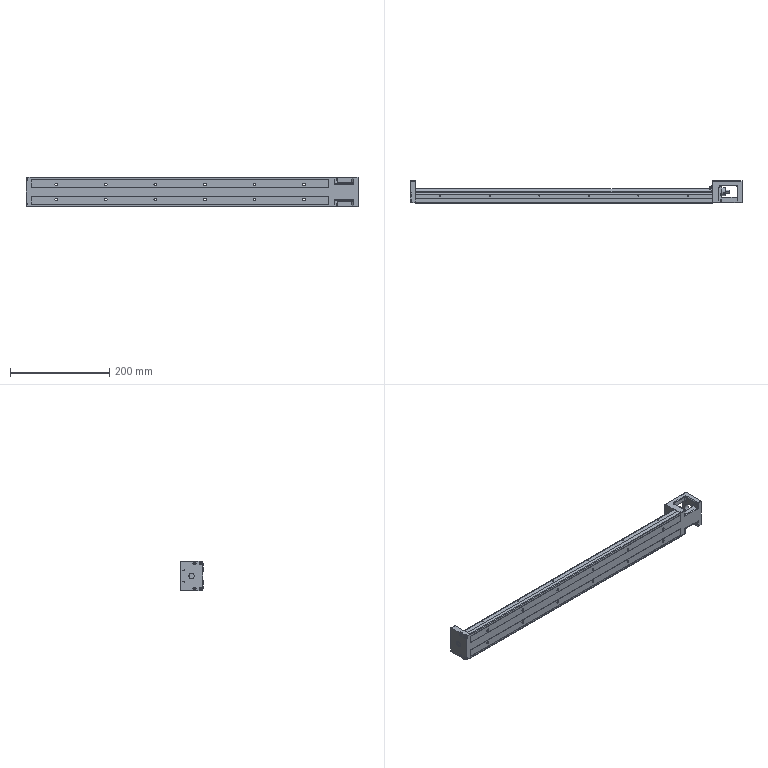Part | STEP file | ASND-0110-KK60-600 | 1 solid | 453 faces | box 670 x 44.5 x 60 mm | volume 591746 mm3 | plane 219 | cylinder 193 | cone 26 | torus 11 | sphere 4 | commonest cylinder face diameters 5.5 x40 3 x27 2.15 x24 9.5 x24 3.3 x16 6 x16